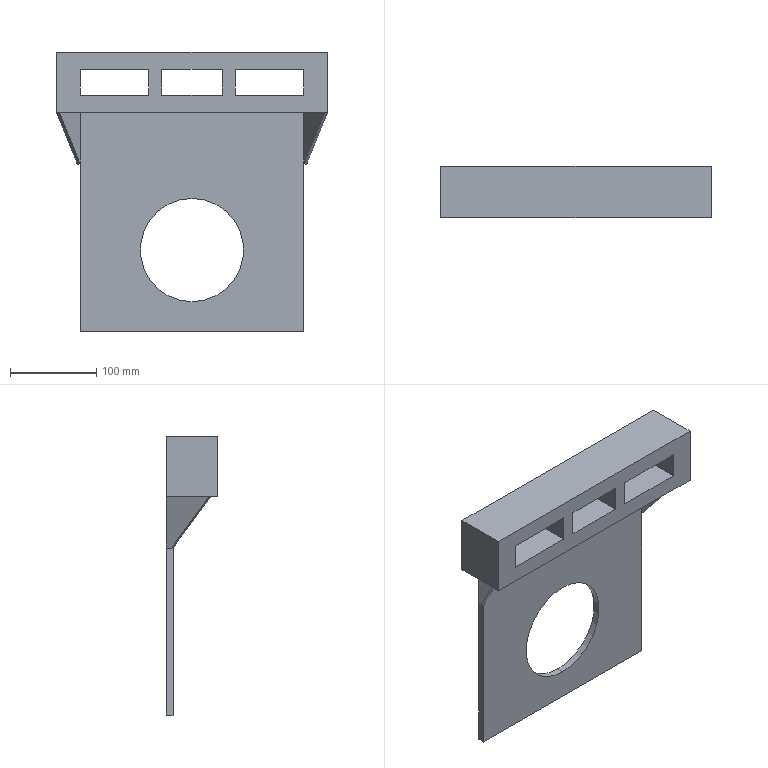Part | SolidWorks | 1 solid | 34 faces | box 315 x 60 x 325 mm | volume 1362122 mm3 | plane 32 | cylinder 2 | commonest cylinder face diameters 120 x2
STEP:
#1=CARTESIAN_POINT('',(0.,8.,-92.5));
#2=VERTEX_POINT('',#1);
#3=CARTESIAN_POINT('',(0.,8.,27.5));
#4=VERTEX_POINT('',#3);
#5=CARTESIAN_POINT('',(0.,8.,-32.5));
#6=DIRECTION('',(0.,1.,0.));
#7=DIRECTION('',(0.,0.,1.));
#8=AXIS2_PLACEMENT_3D('',#5,#6,#7);
#9=CIRCLE('',#8,60.);
#10=EDGE_CURVE('',#2,#4,#9,.T.);
#11=ORIENTED_EDGE('',*,*,#10,.T.);
#12=CARTESIAN_POINT('',(0.,0.,27.5));
#13=VERTEX_POINT('',#12);
#14=CARTESIAN_POINT('',(0.,8.,27.5));
#15=DIRECTION('',(0.,-1.,0.));
#16=VECTOR('',#15,1000.);
#17=LINE('',#14,#16);
#18=EDGE_CURVE('',#4,#13,#17,.T.);
#19=ORIENTED_EDGE('',*,*,#18,.T.);
#20=CARTESIAN_POINT('',(0.,0.,-92.5));
#21=VERTEX_POINT('',#20);
#22=CARTESIAN_POINT('',(0.,0.,-32.5));
#23=DIRECTION('',(0.,1.,0.));
#24=DIRECTION('',(0.,0.,1.));
#25=AXIS2_PLACEMENT_3D('',#22,#23,#24);
#26=CIRCLE('',#25,60.);
#27=EDGE_CURVE('',#21,#13,#26,.T.);
#28=ORIENTED_EDGE('',*,*,#27,.F.);
#29=CARTESIAN_POINT('',(0.,8.,-92.5));
#30=DIRECTION('',(0.,-1.,0.));
#31=VECTOR('',#30,1000.);
#32=LINE('',#29,#31);
#33=EDGE_CURVE('',#2,#21,#32,.T.);
#34=ORIENTED_EDGE('',*,*,#33,.F.);
#35=EDGE_LOOP('',(#11,#19,#28,#34));
#36=FACE_OUTER_BOUND('',#35,.T.);
#37=CARTESIAN_POINT('',(0.,8.,-32.5));
#38=DIRECTION('',(0.,-1.,0.));
#39=DIRECTION('',(0.,0.,-1.));
#40=AXIS2_PLACEMENT_3D('',#37,#38,#39);
#41=CYLINDRICAL_SURFACE('',#40,60.);
#42=ADVANCED_FACE('',(#36),#41,.F.);
#43=CARTESIAN_POINT('',(-154.122,-43.858,127.5));
#44=VERTEX_POINT('',#43);
#45=CARTESIAN_POINT('',(-130.,0.,127.5));
#46=VERTEX_POINT('',#45);
#47=CARTESIAN_POINT('',(-130.,0.,127.5));
#48=DIRECTION('',(0.4819,0.8762,0.));
#49=VECTOR('',#48,1000.);
#50=LINE('',#47,#49);
#51=EDGE_CURVE('',#44,#46,#50,.T.);
#52=ORIENTED_EDGE('',*,*,#51,.F.);
#53=CARTESIAN_POINT('',(-130.,0.,67.5));
#54=VERTEX_POINT('',#53);
#55=CARTESIAN_POINT('',(-130.,0.,67.5));
#56=DIRECTION('',(0.3087,0.5613,-0.7679));
#57=VECTOR('',#56,1000.);
#58=LINE('',#55,#57);
#59=EDGE_CURVE('',#44,#54,#58,.T.);
#60=ORIENTED_EDGE('',*,*,#59,.T.);
#61=CARTESIAN_POINT('',(-130.,0.,67.5));
#62=DIRECTION('',(0.,0.,1.));
#63=VECTOR('',#62,1000.);
#64=LINE('',#61,#63);
#65=EDGE_CURVE('',#54,#46,#64,.T.);
#66=ORIENTED_EDGE('',*,*,#65,.T.);
#67=EDGE_LOOP('',(#52,#60,#66));
#68=FACE_OUTER_BOUND('',#67,.T.);
#69=CARTESIAN_POINT('',(-130.,0.,67.5));
#70=DIRECTION('',(0.8762,-0.4819,0.));
#71=DIRECTION('',(0.4819,0.8762,0.));
#72=AXIS2_PLACEMENT_3D('',#69,#70,#71);
#73=PLANE('',#72);
#74=ADVANCED_FACE('',(#68),#73,.T.);
#75=CARTESIAN_POINT('',(-130.,8.,67.5));
#76=VERTEX_POINT('',#75);
#77=CARTESIAN_POINT('',(-133.378,1.858,67.5));
#78=VERTEX_POINT('',#77);
#79=CARTESIAN_POINT('',(-130.,8.,67.5));
#80=DIRECTION('',(-0.4819,-0.8762,0.));
#81=VECTOR('',#80,1000.);
#82=LINE('',#79,#81);
#83=EDGE_CURVE('',#76,#78,#82,.T.);
#84=ORIENTED_EDGE('',*,*,#83,.T.);
#85=CARTESIAN_POINT('',(-157.5,-42.,127.5));
#86=VERTEX_POINT('',#85);
#87=CARTESIAN_POINT('',(-133.378,1.858,67.5));
#88=DIRECTION('',(-0.3087,-0.5613,0.7679));
#89=VECTOR('',#88,1000.);
#90=LINE('',#87,#89);
#91=EDGE_CURVE('',#78,#86,#90,.T.);
#92=ORIENTED_EDGE('',*,*,#91,.T.);
#93=CARTESIAN_POINT('',(-130.,8.,127.5));
#94=VERTEX_POINT('',#93);
#95=CARTESIAN_POINT('',(-130.,8.,127.5));
#96=DIRECTION('',(-0.4819,-0.8762,0.));
#97=VECTOR('',#96,1000.);
#98=LINE('',#95,#97);
#99=EDGE_CURVE('',#94,#86,#98,.T.);
#100=ORIENTED_EDGE('',*,*,#99,.F.);
#101=CARTESIAN_POINT('',(-130.,8.,67.5));
#102=DIRECTION('',(0.,0.,1.));
#103=VECTOR('',#102,1000.);
#104=LINE('',#101,#103);
#105=EDGE_CURVE('',#76,#94,#104,.T.);
#106=ORIENTED_EDGE('',*,*,#105,.F.);
#107=EDGE_LOOP('',(#84,#92,#100,#106));
#108=FACE_OUTER_BOUND('',#107,.T.);
#109=CARTESIAN_POINT('',(-130.,8.,67.5));
#110=DIRECTION('',(-0.8762,0.4819,0.));
#111=DIRECTION('',(-0.4819,-0.8762,0.));
#112=AXIS2_PLACEMENT_3D('',#109,#110,#111);
#113=PLANE('',#112);
#114=ADVANCED_FACE('',(#108),#113,.T.);
#115=CARTESIAN_POINT('',(-130.,0.,67.5));
#116=DIRECTION('',(0.,1.,0.));
#117=VECTOR('',#116,1000.);
#118=LINE('',#115,#117);
#119=EDGE_CURVE('',#54,#76,#118,.T.);
#120=ORIENTED_EDGE('',*,*,#119,.F.);
#121=CARTESIAN_POINT('',(-30.192,-54.894,67.5));
#122=DIRECTION('',(-0.8762,0.4819,0.));
#123=VECTOR('',#122,1000.);
#124=LINE('',#121,#123);
#125=EDGE_CURVE('',#54,#78,#124,.T.);
#126=ORIENTED_EDGE('',*,*,#125,.T.);
#127=ORIENTED_EDGE('',*,*,#83,.F.);
#128=EDGE_LOOP('',(#120,#126,#127));
#129=FACE_OUTER_BOUND('',#128,.T.);
#130=CARTESIAN_POINT('',(0.,0.,67.5));
#131=DIRECTION('',(0.,0.,-1.));
#132=DIRECTION('',(1.,0.,0.));
#133=AXIS2_PLACEMENT_3D('',#130,#131,#132);
#134=PLANE('',#133);
#135=ADVANCED_FACE('',(#129),#134,.T.);
#136=CARTESIAN_POINT('',(157.5,-52.,127.5));
#137=VERTEX_POINT('',#136);
#138=CARTESIAN_POINT('',(-157.5,-52.,127.5));
#139=VERTEX_POINT('',#138);
#140=CARTESIAN_POINT('',(-157.5,-52.,127.5));
#141=DIRECTION('',(-1.,0.,0.));
#142=VECTOR('',#141,1000.);
#143=LINE('',#140,#142);
#144=EDGE_CURVE('',#137,#139,#143,.T.);
#145=ORIENTED_EDGE('',*,*,#144,.T.);
#146=CARTESIAN_POINT('',(-157.5,-52.,127.5));
#147=DIRECTION('',(0.,1.,0.));
#148=VECTOR('',#147,1000.);
#149=LINE('',#146,#148);
#150=EDGE_CURVE('',#139,#86,#149,.T.);
#151=ORIENTED_EDGE('',*,*,#150,.T.);
#152=CARTESIAN_POINT('',(-154.122,-43.858,127.5));
#153=DIRECTION('',(0.8762,-0.4819,0.));
#154=VECTOR('',#153,1000.);
#155=LINE('',#152,#154);
#156=EDGE_CURVE('',#86,#44,#155,.T.);
#157=ORIENTED_EDGE('',*,*,#156,.T.);
#158=ORIENTED_EDGE('',*,*,#51,.T.);
#159=CARTESIAN_POINT('',(130.,0.,127.5));
#160=VERTEX_POINT('',#159);
#161=CARTESIAN_POINT('',(-130.,0.,127.5));
#162=DIRECTION('',(1.,0.,0.));
#163=VECTOR('',#162,1000.);
#164=LINE('',#161,#163);
#165=EDGE_CURVE('',#46,#160,#164,.T.);
#166=ORIENTED_EDGE('',*,*,#165,.T.);
#167=CARTESIAN_POINT('',(154.122,-43.858,127.5));
#168=VERTEX_POINT('',#167);
#169=CARTESIAN_POINT('',(130.,0.,127.5));
#170=DIRECTION('',(-0.4819,0.8762,0.));
#171=VECTOR('',#170,1000.);
#172=LINE('',#169,#171);
#173=EDGE_CURVE('',#168,#160,#172,.T.);
#174=ORIENTED_EDGE('',*,*,#173,.F.);
#175=CARTESIAN_POINT('',(157.5,-42.,127.5));
#176=VERTEX_POINT('',#175);
#177=CARTESIAN_POINT('',(154.122,-43.858,127.5));
#178=DIRECTION('',(-0.8762,-0.4819,0.));
#179=VECTOR('',#178,1000.);
#180=LINE('',#177,#179);
#181=EDGE_CURVE('',#176,#168,#180,.T.);
#182=ORIENTED_EDGE('',*,*,#181,.F.);
#183=CARTESIAN_POINT('',(157.5,-52.,127.5));
#184=DIRECTION('',(0.,1.,0.));
#185=VECTOR('',#184,1000.);
#186=LINE('',#183,#185);
#187=EDGE_CURVE('',#137,#176,#186,.T.);
#188=ORIENTED_EDGE('',*,*,#187,.F.);
#189=EDGE_LOOP('',(#145,#151,#157,#158,#166,#174,#182,#188));
#190=FACE_OUTER_BOUND('',#189,.T.);
#191=CARTESIAN_POINT('',(-157.5,-52.,127.5));
#192=DIRECTION('',(0.,0.,-1.));
#193=DIRECTION('',(-1.,0.,0.));
#194=AXIS2_PLACEMENT_3D('',#191,#192,#193);
#195=PLANE('',#194);
#196=ADVANCED_FACE('',(#190),#195,.T.);
#197=CARTESIAN_POINT('',(157.5,8.,127.5));
#198=VERTEX_POINT('',#197);
#199=CARTESIAN_POINT('',(157.5,-52.,127.5));
#200=DIRECTION('',(0.,1.,0.));
#201=VECTOR('',#200,1000.);
#202=LINE('',#199,#201);
#203=EDGE_CURVE('',#176,#198,#202,.T.);
#204=ORIENTED_EDGE('',*,*,#203,.F.);
#205=CARTESIAN_POINT('',(130.,8.,127.5));
#206=VERTEX_POINT('',#205);
#207=CARTESIAN_POINT('',(130.,8.,127.5));
#208=DIRECTION('',(0.4819,-0.8762,0.));
#209=VECTOR('',#208,1000.);
#210=LINE('',#207,#209);
#211=EDGE_CURVE('',#206,#176,#210,.T.);
#212=ORIENTED_EDGE('',*,*,#211,.F.);
#213=CARTESIAN_POINT('',(-157.5,8.,127.5));
#214=DIRECTION('',(-1.,0.,0.));
#215=VECTOR('',#214,1000.);
#216=LINE('',#213,#215);
#217=EDGE_CURVE('',#198,#206,#216,.T.);
#218=ORIENTED_EDGE('',*,*,#217,.F.);
#219=EDGE_LOOP('',(#204,#212,#218));
#220=FACE_OUTER_BOUND('',#219,.T.);
#221=CARTESIAN_POINT('',(-157.5,-52.,127.5));
#222=DIRECTION('',(0.,0.,-1.));
#223=DIRECTION('',(-1.,0.,0.));
#224=AXIS2_PLACEMENT_3D('',#221,#222,#223);
#225=PLANE('',#224);
#226=ADVANCED_FACE('',(#220),#225,.T.);
#227=ORIENTED_EDGE('',*,*,#99,.T.);
#228=CARTESIAN_POINT('',(-157.5,8.,127.5));
#229=VERTEX_POINT('',#228);
#230=CARTESIAN_POINT('',(-157.5,-52.,127.5));
#231=DIRECTION('',(0.,1.,0.));
#232=VECTOR('',#231,1000.);
#233=LINE('',#230,#232);
#234=EDGE_CURVE('',#86,#229,#233,.T.);
#235=ORIENTED_EDGE('',*,*,#234,.T.);
#236=CARTESIAN_POINT('',(-157.5,8.,127.5));
#237=DIRECTION('',(-1.,0.,0.));
#238=VECTOR('',#237,1000.);
#239=LINE('',#236,#238);
#240=EDGE_CURVE('',#94,#229,#239,.T.);
#241=ORIENTED_EDGE('',*,*,#240,.F.);
#242=EDGE_LOOP('',(#227,#235,#241));
#243=FACE_OUTER_BOUND('',#242,.T.);
#244=CARTESIAN_POINT('',(-157.5,-52.,127.5));
#245=DIRECTION('',(0.,0.,-1.));
#246=DIRECTION('',(-1.,0.,0.));
#247=AXIS2_PLACEMENT_3D('',#244,#245,#246);
#248=PLANE('',#247);
#249=ADVANCED_FACE('',(#243),#248,.T.);
#250=CARTESIAN_POINT('',(130.,8.,67.5));
#251=VERTEX_POINT('',#250);
#252=CARTESIAN_POINT('',(130.,8.,-127.5));
#253=DIRECTION('',(0.,0.,-1.));
#254=VECTOR('',#253,1000.);
#255=LINE('',#252,#254);
#256=EDGE_CURVE('',#206,#251,#255,.T.);
#257=ORIENTED_EDGE('',*,*,#256,.T.);
#258=CARTESIAN_POINT('',(130.,8.,-127.5));
#259=VERTEX_POINT('',#258);
#260=CARTESIAN_POINT('',(130.,8.,-127.5));
#261=DIRECTION('',(0.,0.,-1.));
#262=VECTOR('',#261,1000.);
#263=LINE('',#260,#262);
#264=EDGE_CURVE('',#251,#259,#263,.T.);
#265=ORIENTED_EDGE('',*,*,#264,.T.);
#266=CARTESIAN_POINT('',(-130.,8.,-127.5));
#267=VERTEX_POINT('',#266);
#268=CARTESIAN_POINT('',(-130.,8.,-127.5));
#269=DIRECTION('',(-1.,0.,0.));
#270=VECTOR('',#269,1000.);
#271=LINE('',#268,#270);
#272=EDGE_CURVE('',#259,#267,#271,.T.);
#273=ORIENTED_EDGE('',*,*,#272,.T.);
#274=CARTESIAN_POINT('',(-130.,8.,-127.5));
#275=DIRECTION('',(0.,0.,1.));
#276=VECTOR('',#275,1000.);
#277=LINE('',#274,#276);
#278=EDGE_CURVE('',#267,#76,#277,.T.);
#279=ORIENTED_EDGE('',*,*,#278,.T.);
#280=ORIENTED_EDGE('',*,*,#105,.T.);
#281=ORIENTED_EDGE('',*,*,#240,.T.);
#282=CARTESIAN_POINT('',(-157.5,8.,197.5));
#283=VERTEX_POINT('',#282);
#284=CARTESIAN_POINT('',(-157.5,8.,197.5));
#285=DIRECTION('',(0.,0.,1.));
#286=VECTOR('',#285,1000.);
#287=LINE('',#284,#286);
#288=EDGE_CURVE('',#229,#283,#287,.T.);
#289=ORIENTED_EDGE('',*,*,#288,.T.);
#290=CARTESIAN_POINT('',(157.5,8.,197.5));
#291=VERTEX_POINT('',#290);
#292=CARTESIAN_POINT('',(-157.5,8.,197.5));
#293=DIRECTION('',(1.,0.,0.));
#294=VECTOR('',#293,1000.);
#295=LINE('',#292,#294);
#296=EDGE_CURVE('',#283,#291,#295,.T.);
#297=ORIENTED_EDGE('',*,*,#296,.T.);
#298=CARTESIAN_POINT('',(157.5,8.,197.5));
#299=DIRECTION('',(0.,0.,-1.));
#300=VECTOR('',#299,1000.);
#301=LINE('',#298,#300);
#302=EDGE_CURVE('',#291,#198,#301,.T.);
#303=ORIENTED_EDGE('',*,*,#302,.T.);
#304=ORIENTED_EDGE('',*,*,#217,.T.);
#305=EDGE_LOOP('',(#257,#265,#273,#279,#280,#281,#289,#297,#303,#304));
#306=FACE_OUTER_BOUND('',#305,.T.);
#307=ORIENTED_EDGE('',*,*,#10,.F.);
#308=CARTESIAN_POINT('',(0.,8.,-32.5));
#309=DIRECTION('',(0.,1.,0.));
#310=DIRECTION('',(0.,0.,1.));
#311=AXIS2_PLACEMENT_3D('',#308,#309,#310);
#312=CIRCLE('',#311,60.);
#313=EDGE_CURVE('',#4,#2,#312,.T.);
#314=ORIENTED_EDGE('',*,*,#313,.F.);
#315=EDGE_LOOP('',(#307,#314));
#316=FACE_BOUND('',#315,.T.);
#317=CARTESIAN_POINT('',(-50.,8.,147.5));
#318=VERTEX_POINT('',#317);
#319=CARTESIAN_POINT('',(-130.,8.,147.5));
#320=VERTEX_POINT('',#319);
#321=CARTESIAN_POINT('',(-130.,8.,147.5));
#322=DIRECTION('',(-1.,0.,0.));
#323=VECTOR('',#322,1000.);
#324=LINE('',#321,#323);
#325=EDGE_CURVE('',#318,#320,#324,.T.);
#326=ORIENTED_EDGE('',*,*,#325,.F.);
#327=CARTESIAN_POINT('',(-50.,8.,177.5));
#328=VERTEX_POINT('',#327);
#329=CARTESIAN_POINT('',(-50.,8.,177.5));
#330=DIRECTION('',(0.,0.,-1.));
#331=VECTOR('',#330,1000.);
#332=LINE('',#329,#331);
#333=EDGE_CURVE('',#328,#318,#332,.T.);
#334=ORIENTED_EDGE('',*,*,#333,.F.);
#335=CARTESIAN_POINT('',(-130.,8.,177.5));
#336=VERTEX_POINT('',#335);
#337=CARTESIAN_POINT('',(-130.,8.,177.5));
#338=DIRECTION('',(1.,0.,0.));
#339=VECTOR('',#338,1000.);
#340=LINE('',#337,#339);
#341=EDGE_CURVE('',#336,#328,#340,.T.);
#342=ORIENTED_EDGE('',*,*,#341,.F.);
#343=CARTESIAN_POINT('',(-130.,8.,177.5));
#344=DIRECTION('',(0.,0.,1.));
#345=VECTOR('',#344,1000.);
#346=LINE('',#343,#345);
#347=EDGE_CURVE('',#320,#336,#346,.T.);
#348=ORIENTED_EDGE('',*,*,#347,.F.);
#349=EDGE_LOOP('',(#326,#334,#342,#348));
#350=FACE_BOUND('',#349,.T.);
#351=CARTESIAN_POINT('',(130.,8.,147.5));
#352=VERTEX_POINT('',#351);
#353=CARTESIAN_POINT('',(50.,8.,147.5));
#354=VERTEX_POINT('',#353);
#355=CARTESIAN_POINT('',(50.,8.,147.5));
#356=DIRECTION('',(-1.,0.,0.));
#357=VECTOR('',#356,1000.);
#358=LINE('',#355,#357);
#359=EDGE_CURVE('',#352,#354,#358,.T.);
#360=ORIENTED_EDGE('',*,*,#359,.F.);
#361=CARTESIAN_POINT('',(130.,8.,177.5));
#362=VERTEX_POINT('',#361);
#363=CARTESIAN_POINT('',(130.,8.,177.5));
#364=DIRECTION('',(0.,0.,-1.));
#365=VECTOR('',#364,1000.);
#366=LINE('',#363,#365);
#367=EDGE_CURVE('',#362,#352,#366,.T.);
#368=ORIENTED_EDGE('',*,*,#367,.F.);
#369=CARTESIAN_POINT('',(50.,8.,177.5));
#370=VERTEX_POINT('',#369);
#371=CARTESIAN_POINT('',(50.,8.,177.5));
#372=DIRECTION('',(1.,0.,0.));
#373=VECTOR('',#372,1000.);
#374=LINE('',#371,#373);
#375=EDGE_CURVE('',#370,#362,#374,.T.);
#376=ORIENTED_EDGE('',*,*,#375,.F.);
#377=CARTESIAN_POINT('',(50.,8.,177.5));
#378=DIRECTION('',(0.,0.,1.));
#379=VECTOR('',#378,1000.);
#380=LINE('',#377,#379);
#381=EDGE_CURVE('',#354,#370,#380,.T.);
#382=ORIENTED_EDGE('',*,*,#381,.F.);
#383=EDGE_LOOP('',(#360,#368,#376,#382));
#384=FACE_BOUND('',#383,.T.);
#385=CARTESIAN_POINT('',(35.,8.,147.5));
#386=VERTEX_POINT('',#385);
#387=CARTESIAN_POINT('',(-35.,8.,147.5));
#388=VERTEX_POINT('',#387);
#389=CARTESIAN_POINT('',(-35.,8.,147.5));
#390=DIRECTION('',(-1.,0.,0.));
#391=VECTOR('',#390,1000.);
#392=LINE('',#389,#391);
#393=EDGE_CURVE('',#386,#388,#392,.T.);
#394=ORIENTED_EDGE('',*,*,#393,.F.);
#395=CARTESIAN_POINT('',(35.,8.,177.5));
#396=VERTEX_POINT('',#395);
#397=CARTESIAN_POINT('',(35.,8.,147.5));
#398=DIRECTION('',(0.,0.,-1.));
#399=VECTOR('',#398,1000.);
#400=LINE('',#397,#399);
#401=EDGE_CURVE('',#396,#386,#400,.T.);
#402=ORIENTED_EDGE('',*,*,#401,.F.);
#403=CARTESIAN_POINT('',(-35.,8.,177.5));
#404=VERTEX_POINT('',#403);
#405=CARTESIAN_POINT('',(-35.,8.,177.5));
#406=DIRECTION('',(1.,0.,0.));
#407=VECTOR('',#406,1000.);
#408=LINE('',#405,#407);
#409=EDGE_CURVE('',#404,#396,#408,.T.);
#410=ORIENTED_EDGE('',*,*,#409,.F.);
#411=CARTESIAN_POINT('',(-35.,8.,147.5));
#412=DIRECTION('',(0.,0.,1.));
#413=VECTOR('',#412,1000.);
#414=LINE('',#411,#413);
#415=EDGE_CURVE('',#388,#404,#414,.T.);
#416=ORIENTED_EDGE('',*,*,#415,.F.);
#417=EDGE_LOOP('',(#394,#402,#410,#416));
#418=FACE_BOUND('',#417,.T.);
#419=CARTESIAN_POINT('',(0.,8.,0.));
#420=DIRECTION('',(0.,1.,0.));
#421=DIRECTION('',(0.,0.,1.));
#422=AXIS2_PLACEMENT_3D('',#419,#420,#421);
#423=PLANE('',#422);
#424=ADVANCED_FACE('',(#306,#316,#350,#384,#418),#423,.T.);
#425=CARTESIAN_POINT('',(130.,0.,67.5));
#426=VERTEX_POINT('',#425);
#427=CARTESIAN_POINT('',(130.,0.,-127.5));
#428=DIRECTION('',(0.,0.,-1.));
#429=VECTOR('',#428,1000.);
#430=LINE('',#427,#429);
#431=EDGE_CURVE('',#160,#426,#430,.T.);
#432=ORIENTED_EDGE('',*,*,#431,.F.);
#433=ORIENTED_EDGE('',*,*,#165,.F.);
#434=ORIENTED_EDGE('',*,*,#65,.F.);
#435=CARTESIAN_POINT('',(-130.,0.,-127.5));
#436=VERTEX_POINT('',#435);
#437=CARTESIAN_POINT('',(-130.,0.,-127.5));
#438=DIRECTION('',(0.,0.,1.));
#439=VECTOR('',#438,1000.);
#440=LINE('',#437,#439);
#441=EDGE_CURVE('',#436,#54,#440,.T.);
#442=ORIENTED_EDGE('',*,*,#441,.F.);
#443=CARTESIAN_POINT('',(130.,0.,-127.5));
#444=VERTEX_POINT('',#443);
#445=CARTESIAN_POINT('',(-130.,0.,-127.5));
#446=DIRECTION('',(-1.,0.,0.));
#447=VECTOR('',#446,1000.);
#448=LINE('',#445,#447);
#449=EDGE_CURVE('',#444,#436,#448,.T.);
#450=ORIENTED_EDGE('',*,*,#449,.F.);
#451=CARTESIAN_POINT('',(130.,0.,-127.5));
#452=DIRECTION('',(0.,0.,-1.));
#453=VECTOR('',#452,1000.);
#454=LINE('',#451,#453);
#455=EDGE_CURVE('',#426,#444,#454,.T.);
#456=ORIENTED_EDGE('',*,*,#455,.F.);
#457=EDGE_LOOP('',(#432,#433,#434,#442,#450,#456));
#458=FACE_OUTER_BOUND('',#457,.T.);
#459=ORIENTED_EDGE('',*,*,#27,.T.);
#460=CARTESIAN_POINT('',(0.,0.,-32.5));
#461=DIRECTION('',(0.,1.,0.));
#462=DIRECTION('',(0.,0.,1.));
#463=AXIS2_PLACEMENT_3D('',#460,#461,#462);
#464=CIRCLE('',#463,60.);
#465=EDGE_CURVE('',#13,#21,#464,.T.);
#466=ORIENTED_EDGE('',*,*,#465,.T.);
#467=EDGE_LOOP('',(#459,#466));
#468=FACE_BOUND('',#467,.T.);
#469=CARTESIAN_POINT('',(0.,0.,0.));
#470=DIRECTION('',(0.,1.,0.));
#471=DIRECTION('',(0.,0.,1.));
#472=AXIS2_PLACEMENT_3D('',#469,#470,#471);
#473=PLANE('',#472);
#474=ADVANCED_FACE('',(#458,#468),#473,.F.);
#475=ORIENTED_EDGE('',*,*,#264,.F.);
#476=CARTESIAN_POINT('',(130.,0.,67.5));
#477=DIRECTION('',(0.,1.,0.));
#478=VECTOR('',#477,1000.);
#479=LINE('',#476,#478);
#480=EDGE_CURVE('',#426,#251,#479,.T.);
#481=ORIENTED_EDGE('',*,*,#480,.F.);
#482=ORIENTED_EDGE('',*,*,#455,.T.);
#483=CARTESIAN_POINT('',(130.,8.,-127.5));
#484=DIRECTION('',(0.,-1.,0.));
#485=VECTOR('',#484,1000.);
#486=LINE('',#483,#485);
#487=EDGE_CURVE('',#259,#444,#486,.T.);
#488=ORIENTED_EDGE('',*,*,#487,.F.);
#489=EDGE_LOOP('',(#475,#481,#482,#488));
#490=FACE_OUTER_BOUND('',#489,.T.);
#491=CARTESIAN_POINT('',(130.,8.,-127.5));
#492=DIRECTION('',(-1.,0.,0.));
#493=DIRECTION('',(0.,0.,1.));
#494=AXIS2_PLACEMENT_3D('',#491,#492,#493);
#495=PLANE('',#494);
#496=ADVANCED_FACE('',(#490),#495,.F.);
#497=ORIENTED_EDGE('',*,*,#449,.T.);
#498=CARTESIAN_POINT('',(-130.,8.,-127.5));
#499=DIRECTION('',(0.,-1.,0.));
#500=VECTOR('',#499,1000.);
#501=LINE('',#498,#500);
#502=EDGE_CURVE('',#267,#436,#501,.T.);
#503=ORIENTED_EDGE('',*,*,#502,.F.);
#504=ORIENTED_EDGE('',*,*,#272,.F.);
#505=ORIENTED_EDGE('',*,*,#487,.T.);
#506=EDGE_LOOP('',(#497,#503,#504,#505));
#507=FACE_OUTER_BOUND('',#506,.T.);
#508=CARTESIAN_POINT('',(-130.,8.,-127.5));
#509=DIRECTION('',(0.,0.,1.));
#510=DIRECTION('',(1.,0.,0.));
#511=AXIS2_PLACEMENT_3D('',#508,#509,#510);
#512=PLANE('',#511);
#513=ADVANCED_FACE('',(#507),#512,.F.);
#514=ORIENTED_EDGE('',*,*,#441,.T.);
#515=ORIENTED_EDGE('',*,*,#119,.T.);
#516=ORIENTED_EDGE('',*,*,#278,.F.);
#517=ORIENTED_EDGE('',*,*,#502,.T.);
#518=EDGE_LOOP('',(#514,#515,#516,#517));
#519=FACE_OUTER_BOUND('',#518,.T.);
#520=CARTESIAN_POINT('',(-130.,8.,-127.5));
#521=DIRECTION('',(1.,0.,0.));
#522=DIRECTION('',(0.,0.,-1.));
#523=AXIS2_PLACEMENT_3D('',#520,#521,#522);
#524=PLANE('',#523);
#525=ADVANCED_FACE('',(#519),#524,.F.);
#526=ORIENTED_EDGE('',*,*,#18,.F.);
#527=ORIENTED_EDGE('',*,*,#313,.T.);
#528=ORIENTED_EDGE('',*,*,#33,.T.);
#529=ORIENTED_EDGE('',*,*,#465,.F.);
#530=EDGE_LOOP('',(#526,#527,#528,#529));
#531=FACE_OUTER_BOUND('',#530,.T.);
#532=CARTESIAN_POINT('',(0.,8.,-32.5));
#533=DIRECTION('',(0.,-1.,0.));
#534=DIRECTION('',(0.,0.,-1.));
#535=AXIS2_PLACEMENT_3D('',#532,#533,#534);
#536=CYLINDRICAL_SURFACE('',#535,60.);
#537=ADVANCED_FACE('',(#531),#536,.F.);
#538=ORIENTED_EDGE('',*,*,#302,.F.);
#539=CARTESIAN_POINT('',(157.5,-52.,197.5));
#540=VERTEX_POINT('',#539);
#541=CARTESIAN_POINT('',(157.5,-52.,197.5));
#542=DIRECTION('',(0.,1.,0.));
#543=VECTOR('',#542,1000.);
#544=LINE('',#541,#543);
#545=EDGE_CURVE('',#540,#291,#544,.T.);
#546=ORIENTED_EDGE('',*,*,#545,.F.);
#547=CARTESIAN_POINT('',(157.5,-52.,197.5));
#548=DIRECTION('',(0.,0.,-1.));
#549=VECTOR('',#548,1000.);
#550=LINE('',#547,#549);
#551=EDGE_CURVE('',#540,#137,#550,.T.);
#552=ORIENTED_EDGE('',*,*,#551,.T.);
#553=ORIENTED_EDGE('',*,*,#187,.T.);
#554=ORIENTED_EDGE('',*,*,#203,.T.);
#555=EDGE_LOOP('',(#538,#546,#552,#553,#554));
#556=FACE_OUTER_BOUND('',#555,.T.);
#557=CARTESIAN_POINT('',(157.5,-52.,197.5));
#558=DIRECTION('',(1.,0.,0.));
#559=DIRECTION('',(0.,0.,-1.));
#560=AXIS2_PLACEMENT_3D('',#557,#558,#559);
#561=PLANE('',#560);
#562=ADVANCED_FACE('',(#556),#561,.T.);
#563=ORIENTED_EDGE('',*,*,#296,.F.);
#564=CARTESIAN_POINT('',(-157.5,-52.,197.5));
#565=VERTEX_POINT('',#564);
#566=CARTESIAN_POINT('',(-157.5,-52.,197.5));
#567=DIRECTION('',(0.,1.,0.));
#568=VECTOR('',#567,1000.);
#569=LINE('',#566,#568);
#570=EDGE_CURVE('',#565,#283,#569,.T.);
#571=ORIENTED_EDGE('',*,*,#570,.F.);
#572=CARTESIAN_POINT('',(-157.5,-52.,197.5));
#573=DIRECTION('',(1.,0.,0.));
#574=VECTOR('',#573,1000.);
#575=LINE('',#572,#574);
#576=EDGE_CURVE('',#565,#540,#575,.T.);
#577=ORIENTED_EDGE('',*,*,#576,.T.);
#578=ORIENTED_EDGE('',*,*,#545,.T.);
#579=EDGE_LOOP('',(#563,#571,#577,#578));
#580=FACE_OUTER_BOUND('',#579,.T.);
#581=CARTESIAN_POINT('',(-157.5,-52.,197.5));
#582=DIRECTION('',(0.,0.,1.));
#583=DIRECTION('',(1.,0.,0.));
#584=AXIS2_PLACEMENT_3D('',#581,#582,#583);
#585=PLANE('',#584);
#586=ADVANCED_FACE('',(#580),#585,.T.);
#587=ORIENTED_EDGE('',*,*,#288,.F.);
#588=ORIENTED_EDGE('',*,*,#234,.F.);
#589=ORIENTED_EDGE('',*,*,#150,.F.);
#590=CARTESIAN_POINT('',(-157.5,-52.,197.5));
#591=DIRECTION('',(0.,0.,1.));
#592=VECTOR('',#591,1000.);
#593=LINE('',#590,#592);
#594=EDGE_CURVE('',#139,#565,#593,.T.);
#595=ORIENTED_EDGE('',*,*,#594,.T.);
#596=ORIENTED_EDGE('',*,*,#570,.T.);
#597=EDGE_LOOP('',(#587,#588,#589,#595,#596));
#598=FACE_OUTER_BOUND('',#597,.T.);
#599=CARTESIAN_POINT('',(-157.5,-52.,197.5));
#600=DIRECTION('',(-1.,0.,0.));
#601=DIRECTION('',(0.,0.,1.));
#602=AXIS2_PLACEMENT_3D('',#599,#600,#601);
#603=PLANE('',#602);
#604=ADVANCED_FACE('',(#598),#603,.T.);
#605=CARTESIAN_POINT('',(-50.,-52.,177.5));
#606=VERTEX_POINT('',#605);
#607=CARTESIAN_POINT('',(-50.,-52.,147.5));
#608=VERTEX_POINT('',#607);
#609=CARTESIAN_POINT('',(-50.,-52.,177.5));
#610=DIRECTION('',(0.,0.,-1.));
#611=VECTOR('',#610,1000.);
#612=LINE('',#609,#611);
#613=EDGE_CURVE('',#606,#608,#612,.T.);
#614=ORIENTED_EDGE('',*,*,#613,.T.);
#615=CARTESIAN_POINT('',(-130.,-52.,147.5));
#616=VERTEX_POINT('',#615);
#617=CARTESIAN_POINT('',(-130.,-52.,147.5));
#618=DIRECTION('',(-1.,0.,0.));
#619=VECTOR('',#618,1000.);
#620=LINE('',#617,#619);
#621=EDGE_CURVE('',#608,#616,#620,.T.);
#622=ORIENTED_EDGE('',*,*,#621,.T.);
#623=CARTESIAN_POINT('',(-130.,-52.,177.5));
#624=VERTEX_POINT('',#623);
#625=CARTESIAN_POINT('',(-130.,-52.,177.5));
#626=DIRECTION('',(0.,0.,1.));
#627=VECTOR('',#626,1000.);
#628=LINE('',#625,#627);
#629=EDGE_CURVE('',#616,#624,#628,.T.);
#630=ORIENTED_EDGE('',*,*,#629,.T.);
#631=CARTESIAN_POINT('',(-130.,-52.,177.5));
#632=DIRECTION('',(1.,0.,0.));
#633=VECTOR('',#632,1000.);
#634=LINE('',#631,#633);
#635=EDGE_CURVE('',#624,#606,#634,.T.);
#636=ORIENTED_EDGE('',*,*,#635,.T.);
#637=EDGE_LOOP('',(#614,#622,#630,#636));
#638=FACE_BOUND('',#637,.T.);
#639=CARTESIAN_POINT('',(130.,-52.,177.5));
#640=VERTEX_POINT('',#639);
#641=CARTESIAN_POINT('',(130.,-52.,147.5));
#642=VERTEX_POINT('',#641);
#643=CARTESIAN_POINT('',(130.,-52.,177.5));
#644=DIRECTION('',(0.,0.,-1.));
#645=VECTOR('',#644,1000.);
#646=LINE('',#643,#645);
#647=EDGE_CURVE('',#640,#642,#646,.T.);
#648=ORIENTED_EDGE('',*,*,#647,.T.);
#649=CARTESIAN_POINT('',(50.,-52.,147.5));
#650=VERTEX_POINT('',#649);
#651=CARTESIAN_POINT('',(50.,-52.,147.5));
#652=DIRECTION('',(-1.,0.,0.));
#653=VECTOR('',#652,1000.);
#654=LINE('',#651,#653);
#655=EDGE_CURVE('',#642,#650,#654,.T.);
#656=ORIENTED_EDGE('',*,*,#655,.T.);
#657=CARTESIAN_POINT('',(50.,-52.,177.5));
#658=VERTEX_POINT('',#657);
#659=CARTESIAN_POINT('',(50.,-52.,177.5));
#660=DIRECTION('',(0.,0.,1.));
#661=VECTOR('',#660,1000.);
#662=LINE('',#659,#661);
#663=EDGE_CURVE('',#650,#658,#662,.T.);
#664=ORIENTED_EDGE('',*,*,#663,.T.);
#665=CARTESIAN_POINT('',(50.,-52.,177.5));
#666=DIRECTION('',(1.,0.,0.));
#667=VECTOR('',#666,1000.);
#668=LINE('',#665,#667);
#669=EDGE_CURVE('',#658,#640,#668,.T.);
#670=ORIENTED_EDGE('',*,*,#669,.T.);
#671=EDGE_LOOP('',(#648,#656,#664,#670));
#672=FACE_BOUND('',#671,.T.);
#673=CARTESIAN_POINT('',(35.,-52.,177.5));
#674=VERTEX_POINT('',#673);
#675=CARTESIAN_POINT('',(35.,-52.,147.5));
#676=VERTEX_POINT('',#675);
#677=CARTESIAN_POINT('',(35.,-52.,147.5));
#678=DIRECTION('',(0.,0.,-1.));
#679=VECTOR('',#678,1000.);
#680=LINE('',#677,#679);
#681=EDGE_CURVE('',#674,#676,#680,.T.);
#682=ORIENTED_EDGE('',*,*,#681,.T.);
#683=CARTESIAN_POINT('',(-35.,-52.,147.5));
#684=VERTEX_POINT('',#683);
#685=CARTESIAN_POINT('',(-35.,-52.,147.5));
#686=DIRECTION('',(-1.,0.,0.));
#687=VECTOR('',#686,1000.);
#688=LINE('',#685,#687);
#689=EDGE_CURVE('',#676,#684,#688,.T.);
#690=ORIENTED_EDGE('',*,*,#689,.T.);
#691=CARTESIAN_POINT('',(-35.,-52.,177.5));
#692=VERTEX_POINT('',#691);
#693=CARTESIAN_POINT('',(-35.,-52.,147.5));
#694=DIRECTION('',(0.,0.,1.));
#695=VECTOR('',#694,1000.);
#696=LINE('',#693,#695);
#697=EDGE_CURVE('',#684,#692,#696,.T.);
#698=ORIENTED_EDGE('',*,*,#697,.T.);
#699=CARTESIAN_POINT('',(-35.,-52.,177.5));
#700=DIRECTION('',(1.,0.,0.));
#701=VECTOR('',#700,1000.);
#702=LINE('',#699,#701);
#703=EDGE_CURVE('',#692,#674,#702,.T.);
#704=ORIENTED_EDGE('',*,*,#703,.T.);
#705=EDGE_LOOP('',(#682,#690,#698,#704));
#706=FACE_BOUND('',#705,.T.);
#707=ORIENTED_EDGE('',*,*,#551,.F.);
#708=ORIENTED_EDGE('',*,*,#576,.F.);
#709=ORIENTED_EDGE('',*,*,#594,.F.);
#710=ORIENTED_EDGE('',*,*,#144,.F.);
#711=EDGE_LOOP('',(#707,#708,#709,#710));
#712=FACE_OUTER_BOUND('',#711,.T.);
#713=CARTESIAN_POINT('',(0.,-52.,0.));
#714=DIRECTION('',(0.,-1.,0.));
#715=DIRECTION('',(0.,0.,-1.));
#716=AXIS2_PLACEMENT_3D('',#713,#714,#715);
#717=PLANE('',#716);
#718=ADVANCED_FACE('',(#638,#672,#706,#712),#717,.T.);
#719=ORIENTED_EDGE('',*,*,#401,.T.);
#720=CARTESIAN_POINT('',(35.,-52.,147.5));
#721=DIRECTION('',(0.,1.,0.));
#722=VECTOR('',#721,1000.);
#723=LINE('',#720,#722);
#724=EDGE_CURVE('',#676,#386,#723,.T.);
#725=ORIENTED_EDGE('',*,*,#724,.F.);
#726=ORIENTED_EDGE('',*,*,#681,.F.);
#727=CARTESIAN_POINT('',(35.,-52.,177.5));
#728=DIRECTION('',(0.,1.,0.));
#729=VECTOR('',#728,1000.);
#730=LINE('',#727,#729);
#731=EDGE_CURVE('',#674,#396,#730,.T.);
#732=ORIENTED_EDGE('',*,*,#731,.T.);
#733=EDGE_LOOP('',(#719,#725,#726,#732));
#734=FACE_OUTER_BOUND('',#733,.T.);
#735=CARTESIAN_POINT('',(35.,-52.,147.5));
#736=DIRECTION('',(1.,0.,0.));
#737=DIRECTION('',(0.,0.,-1.));
#738=AXIS2_PLACEMENT_3D('',#735,#736,#737);
#739=PLANE('',#738);
#740=ADVANCED_FACE('',(#734),#739,.F.);
#741=ORIENTED_EDGE('',*,*,#409,.T.);
#742=ORIENTED_EDGE('',*,*,#731,.F.);
#743=ORIENTED_EDGE('',*,*,#703,.F.);
#744=CARTESIAN_POINT('',(-35.,-52.,177.5));
#745=DIRECTION('',(0.,1.,0.));
#746=VECTOR('',#745,1000.);
#747=LINE('',#744,#746);
#748=EDGE_CURVE('',#692,#404,#747,.T.);
#749=ORIENTED_EDGE('',*,*,#748,.T.);
#750=EDGE_LOOP('',(#741,#742,#743,#749));
#751=FACE_OUTER_BOUND('',#750,.T.);
#752=CARTESIAN_POINT('',(-35.,-52.,177.5));
#753=DIRECTION('',(0.,0.,1.));
#754=DIRECTION('',(1.,0.,0.));
#755=AXIS2_PLACEMENT_3D('',#752,#753,#754);
#756=PLANE('',#755);
#757=ADVANCED_FACE('',(#751),#756,.F.);
#758=ORIENTED_EDGE('',*,*,#415,.T.);
#759=ORIENTED_EDGE('',*,*,#748,.F.);
#760=ORIENTED_EDGE('',*,*,#697,.F.);
#761=CARTESIAN_POINT('',(-35.,-52.,147.5));
#762=DIRECTION('',(0.,1.,0.));
#763=VECTOR('',#762,1000.);
#764=LINE('',#761,#763);
#765=EDGE_CURVE('',#684,#388,#764,.T.);
#766=ORIENTED_EDGE('',*,*,#765,.T.);
#767=EDGE_LOOP('',(#758,#759,#760,#766));
#768=FACE_OUTER_BOUND('',#767,.T.);
#769=CARTESIAN_POINT('',(-35.,-52.,147.5));
#770=DIRECTION('',(-1.,0.,0.));
#771=DIRECTION('',(0.,0.,1.));
#772=AXIS2_PLACEMENT_3D('',#769,#770,#771);
#773=PLANE('',#772);
#774=ADVANCED_FACE('',(#768),#773,.F.);
#775=ORIENTED_EDGE('',*,*,#393,.T.);
#776=ORIENTED_EDGE('',*,*,#765,.F.);
#777=ORIENTED_EDGE('',*,*,#689,.F.);
#778=ORIENTED_EDGE('',*,*,#724,.T.);
#779=EDGE_LOOP('',(#775,#776,#777,#778));
#780=FACE_OUTER_BOUND('',#779,.T.);
#781=CARTESIAN_POINT('',(-35.,-52.,147.5));
#782=DIRECTION('',(0.,0.,-1.));
#783=DIRECTION('',(-1.,0.,0.));
#784=AXIS2_PLACEMENT_3D('',#781,#782,#783);
#785=PLANE('',#784);
#786=ADVANCED_FACE('',(#780),#785,.F.);
#787=ORIENTED_EDGE('',*,*,#367,.T.);
#788=CARTESIAN_POINT('',(130.,-52.,147.5));
#789=DIRECTION('',(0.,1.,0.));
#790=VECTOR('',#789,1000.);
#791=LINE('',#788,#790);
#792=EDGE_CURVE('',#642,#352,#791,.T.);
#793=ORIENTED_EDGE('',*,*,#792,.F.);
#794=ORIENTED_EDGE('',*,*,#647,.F.);
#795=CARTESIAN_POINT('',(130.,-52.,177.5));
#796=DIRECTION('',(0.,1.,0.));
#797=VECTOR('',#796,1000.);
#798=LINE('',#795,#797);
#799=EDGE_CURVE('',#640,#362,#798,.T.);
#800=ORIENTED_EDGE('',*,*,#799,.T.);
#801=EDGE_LOOP('',(#787,#793,#794,#800));
#802=FACE_OUTER_BOUND('',#801,.T.);
#803=CARTESIAN_POINT('',(130.,-52.,177.5));
#804=DIRECTION('',(1.,0.,0.));
#805=DIRECTION('',(0.,0.,-1.));
#806=AXIS2_PLACEMENT_3D('',#803,#804,#805);
#807=PLANE('',#806);
#808=ADVANCED_FACE('',(#802),#807,.F.);
#809=ORIENTED_EDGE('',*,*,#375,.T.);
#810=ORIENTED_EDGE('',*,*,#799,.F.);
#811=ORIENTED_EDGE('',*,*,#669,.F.);
#812=CARTESIAN_POINT('',(50.,-52.,177.5));
#813=DIRECTION('',(0.,1.,0.));
#814=VECTOR('',#813,1000.);
#815=LINE('',#812,#814);
#816=EDGE_CURVE('',#658,#370,#815,.T.);
#817=ORIENTED_EDGE('',*,*,#816,.T.);
#818=EDGE_LOOP('',(#809,#810,#811,#817));
#819=FACE_OUTER_BOUND('',#818,.T.);
#820=CARTESIAN_POINT('',(50.,-52.,177.5));
#821=DIRECTION('',(0.,0.,1.));
#822=DIRECTION('',(1.,0.,0.));
#823=AXIS2_PLACEMENT_3D('',#820,#821,#822);
#824=PLANE('',#823);
#825=ADVANCED_FACE('',(#819),#824,.F.);
#826=ORIENTED_EDGE('',*,*,#381,.T.);
#827=ORIENTED_EDGE('',*,*,#816,.F.);
#828=ORIENTED_EDGE('',*,*,#663,.F.);
#829=CARTESIAN_POINT('',(50.,-52.,147.5));
#830=DIRECTION('',(0.,1.,0.));
#831=VECTOR('',#830,1000.);
#832=LINE('',#829,#831);
#833=EDGE_CURVE('',#650,#354,#832,.T.);
#834=ORIENTED_EDGE('',*,*,#833,.T.);
#835=EDGE_LOOP('',(#826,#827,#828,#834));
#836=FACE_OUTER_BOUND('',#835,.T.);
#837=CARTESIAN_POINT('',(50.,-52.,177.5));
#838=DIRECTION('',(-1.,0.,0.));
#839=DIRECTION('',(0.,0.,1.));
#840=AXIS2_PLACEMENT_3D('',#837,#838,#839);
#841=PLANE('',#840);
#842=ADVANCED_FACE('',(#836),#841,.F.);
#843=ORIENTED_EDGE('',*,*,#359,.T.);
#844=ORIENTED_EDGE('',*,*,#833,.F.);
#845=ORIENTED_EDGE('',*,*,#655,.F.);
#846=ORIENTED_EDGE('',*,*,#792,.T.);
#847=EDGE_LOOP('',(#843,#844,#845,#846));
#848=FACE_OUTER_BOUND('',#847,.T.);
#849=CARTESIAN_POINT('',(50.,-52.,147.5));
#850=DIRECTION('',(0.,0.,-1.));
#851=DIRECTION('',(-1.,0.,0.));
#852=AXIS2_PLACEMENT_3D('',#849,#850,#851);
#853=PLANE('',#852);
#854=ADVANCED_FACE('',(#848),#853,.F.);
#855=ORIENTED_EDGE('',*,*,#333,.T.);
#856=CARTESIAN_POINT('',(-50.,-52.,147.5));
#857=DIRECTION('',(0.,1.,0.));
#858=VECTOR('',#857,1000.);
#859=LINE('',#856,#858);
#860=EDGE_CURVE('',#608,#318,#859,.T.);
#861=ORIENTED_EDGE('',*,*,#860,.F.);
#862=ORIENTED_EDGE('',*,*,#613,.F.);
#863=CARTESIAN_POINT('',(-50.,-52.,177.5));
#864=DIRECTION('',(0.,1.,0.));
#865=VECTOR('',#864,1000.);
#866=LINE('',#863,#865);
#867=EDGE_CURVE('',#606,#328,#866,.T.);
#868=ORIENTED_EDGE('',*,*,#867,.T.);
#869=EDGE_LOOP('',(#855,#861,#862,#868));
#870=FACE_OUTER_BOUND('',#869,.T.);
#871=CARTESIAN_POINT('',(-50.,-52.,177.5));
#872=DIRECTION('',(1.,0.,0.));
#873=DIRECTION('',(0.,0.,-1.));
#874=AXIS2_PLACEMENT_3D('',#871,#872,#873);
#875=PLANE('',#874);
#876=ADVANCED_FACE('',(#870),#875,.F.);
#877=ORIENTED_EDGE('',*,*,#341,.T.);
#878=ORIENTED_EDGE('',*,*,#867,.F.);
#879=ORIENTED_EDGE('',*,*,#635,.F.);
#880=CARTESIAN_POINT('',(-130.,-52.,177.5));
#881=DIRECTION('',(0.,1.,0.));
#882=VECTOR('',#881,1000.);
#883=LINE('',#880,#882);
#884=EDGE_CURVE('',#624,#336,#883,.T.);
#885=ORIENTED_EDGE('',*,*,#884,.T.);
#886=EDGE_LOOP('',(#877,#878,#879,#885));
#887=FACE_OUTER_BOUND('',#886,.T.);
#888=CARTESIAN_POINT('',(-130.,-52.,177.5));
#889=DIRECTION('',(0.,0.,1.));
#890=DIRECTION('',(1.,0.,0.));
#891=AXIS2_PLACEMENT_3D('',#888,#889,#890);
#892=PLANE('',#891);
#893=ADVANCED_FACE('',(#887),#892,.F.);
#894=ORIENTED_EDGE('',*,*,#347,.T.);
#895=ORIENTED_EDGE('',*,*,#884,.F.);
#896=ORIENTED_EDGE('',*,*,#629,.F.);
#897=CARTESIAN_POINT('',(-130.,-52.,147.5));
#898=DIRECTION('',(0.,1.,0.));
#899=VECTOR('',#898,1000.);
#900=LINE('',#897,#899);
#901=EDGE_CURVE('',#616,#320,#900,.T.);
#902=ORIENTED_EDGE('',*,*,#901,.T.);
#903=EDGE_LOOP('',(#894,#895,#896,#902));
#904=FACE_OUTER_BOUND('',#903,.T.);
#905=CARTESIAN_POINT('',(-130.,-52.,177.5));
#906=DIRECTION('',(-1.,0.,0.));
#907=DIRECTION('',(0.,0.,1.));
#908=AXIS2_PLACEMENT_3D('',#905,#906,#907);
#909=PLANE('',#908);
#910=ADVANCED_FACE('',(#904),#909,.F.);
#911=ORIENTED_EDGE('',*,*,#325,.T.);
#912=ORIENTED_EDGE('',*,*,#901,.F.);
#913=ORIENTED_EDGE('',*,*,#621,.F.);
#914=ORIENTED_EDGE('',*,*,#860,.T.);
#915=EDGE_LOOP('',(#911,#912,#913,#914));
#916=FACE_OUTER_BOUND('',#915,.T.);
#917=CARTESIAN_POINT('',(-130.,-52.,147.5));
#918=DIRECTION('',(0.,0.,-1.));
#919=DIRECTION('',(-1.,0.,0.));
#920=AXIS2_PLACEMENT_3D('',#917,#918,#919);
#921=PLANE('',#920);
#922=ADVANCED_FACE('',(#916),#921,.F.);
#923=ORIENTED_EDGE('',*,*,#211,.T.);
#924=CARTESIAN_POINT('',(133.378,1.858,67.5));
#925=VERTEX_POINT('',#924);
#926=CARTESIAN_POINT('',(133.378,1.858,67.5));
#927=DIRECTION('',(0.3087,-0.5613,0.7679));
#928=VECTOR('',#927,1000.);
#929=LINE('',#926,#928);
#930=EDGE_CURVE('',#925,#176,#929,.T.);
#931=ORIENTED_EDGE('',*,*,#930,.F.);
#932=CARTESIAN_POINT('',(130.,8.,67.5));
#933=DIRECTION('',(0.4819,-0.8762,0.));
#934=VECTOR('',#933,1000.);
#935=LINE('',#932,#934);
#936=EDGE_CURVE('',#251,#925,#935,.T.);
#937=ORIENTED_EDGE('',*,*,#936,.F.);
#938=ORIENTED_EDGE('',*,*,#256,.F.);
#939=EDGE_LOOP('',(#923,#931,#937,#938));
#940=FACE_OUTER_BOUND('',#939,.T.);
#941=CARTESIAN_POINT('',(130.,8.,67.5));
#942=DIRECTION('',(-0.8762,-0.4819,0.));
#943=DIRECTION('',(0.4819,-0.8762,0.));
#944=AXIS2_PLACEMENT_3D('',#941,#942,#943);
#945=PLANE('',#944);
#946=ADVANCED_FACE('',(#940),#945,.F.);
#947=ORIENTED_EDGE('',*,*,#431,.T.);
#948=CARTESIAN_POINT('',(130.,0.,67.5));
#949=DIRECTION('',(0.3087,-0.5613,0.7679));
#950=VECTOR('',#949,1000.);
#951=LINE('',#948,#950);
#952=EDGE_CURVE('',#426,#168,#951,.T.);
#953=ORIENTED_EDGE('',*,*,#952,.T.);
#954=ORIENTED_EDGE('',*,*,#173,.T.);
#955=EDGE_LOOP('',(#947,#953,#954));
#956=FACE_OUTER_BOUND('',#955,.T.);
#957=CARTESIAN_POINT('',(130.,0.,67.5));
#958=DIRECTION('',(0.8762,0.4819,0.));
#959=DIRECTION('',(-0.4819,0.8762,0.));
#960=AXIS2_PLACEMENT_3D('',#957,#958,#959);
#961=PLANE('',#960);
#962=ADVANCED_FACE('',(#956),#961,.F.);
#963=CARTESIAN_POINT('',(30.192,-54.894,67.5));
#964=DIRECTION('',(0.8762,0.4819,0.));
#965=VECTOR('',#964,1000.);
#966=LINE('',#963,#965);
#967=EDGE_CURVE('',#426,#925,#966,.T.);
#968=ORIENTED_EDGE('',*,*,#967,.F.);
#969=ORIENTED_EDGE('',*,*,#480,.T.);
#970=ORIENTED_EDGE('',*,*,#936,.T.);
#971=EDGE_LOOP('',(#968,#969,#970));
#972=FACE_OUTER_BOUND('',#971,.T.);
#973=CARTESIAN_POINT('',(0.,0.,67.5));
#974=DIRECTION('',(0.,0.,-1.));
#975=DIRECTION('',(-1.,0.,0.));
#976=AXIS2_PLACEMENT_3D('',#973,#974,#975);
#977=PLANE('',#976);
#978=ADVANCED_FACE('',(#972),#977,.T.);
#979=ORIENTED_EDGE('',*,*,#967,.T.);
#980=ORIENTED_EDGE('',*,*,#930,.T.);
#981=ORIENTED_EDGE('',*,*,#181,.T.);
#982=ORIENTED_EDGE('',*,*,#952,.F.);
#983=EDGE_LOOP('',(#979,#980,#981,#982));
#984=FACE_OUTER_BOUND('',#983,.T.);
#985=CARTESIAN_POINT('',(80.805,-27.057,67.5));
#986=DIRECTION('',(-0.3701,0.6728,0.6406));
#987=DIRECTION('',(0.,-0.6895,0.7242));
#988=AXIS2_PLACEMENT_3D('',#985,#986,#987);
#989=PLANE('',#988);
#990=ADVANCED_FACE('',(#984),#989,.F.);
#991=ORIENTED_EDGE('',*,*,#156,.F.);
#992=ORIENTED_EDGE('',*,*,#91,.F.);
#993=ORIENTED_EDGE('',*,*,#125,.F.);
#994=ORIENTED_EDGE('',*,*,#59,.F.);
#995=EDGE_LOOP('',(#991,#992,#993,#994));
#996=FACE_OUTER_BOUND('',#995,.T.);
#997=CARTESIAN_POINT('',(-80.805,-27.057,67.5));
#998=DIRECTION('',(-0.3701,-0.6728,-0.6406));
#999=DIRECTION('',(0.,0.6895,-0.7242));
#1000=AXIS2_PLACEMENT_3D('',#997,#998,#999);
#1001=PLANE('',#1000);
#1002=ADVANCED_FACE('',(#996),#1001,.T.);
#1003=CLOSED_SHELL('',(#42,#74,#114,#135,#196,#226,#249,#424,#474,#496,#513,#525,#537,#562,#586,#604,#718,#740,#757,#774,#786,#808,#825,#842,#854,#876,#893,#910,#922,#946,#962,#978,#990,#1002));
#1004=MANIFOLD_SOLID_BREP('',#1003);
#1005=CARTESIAN_POINT('',(0.,0.,0.));
#1006=DIRECTION('',(0.,0.,1.));
#1007=DIRECTION('',(1.,0.,0.));
#1008=AXIS2_PLACEMENT_3D('',#1005,#1006,#1007);
#1009=(LENGTH_UNIT()NAMED_UNIT(*)SI_UNIT(.MILLI.,.METRE.));
#1010=UNCERTAINTY_MEASURE_WITH_UNIT(LENGTH_MEASURE(0.00001),#1009,'','');
#1011=(NAMED_UNIT(*)PLANE_ANGLE_UNIT()SI_UNIT($,.RADIAN.));
#1012=(NAMED_UNIT(*)SI_UNIT($,.STERADIAN.)SOLID_ANGLE_UNIT());
#1013=(GEOMETRIC_REPRESENTATION_CONTEXT(3)GLOBAL_UNCERTAINTY_ASSIGNED_CONTEXT((#1010))GLOBAL_UNIT_ASSIGNED_CONTEXT((#1009,#1011,#1012))REPRESENTATION_CONTEXT('',''));
#1014=ADVANCED_BREP_SHAPE_REPRESENTATION('',(#1004,#1008),#1013);